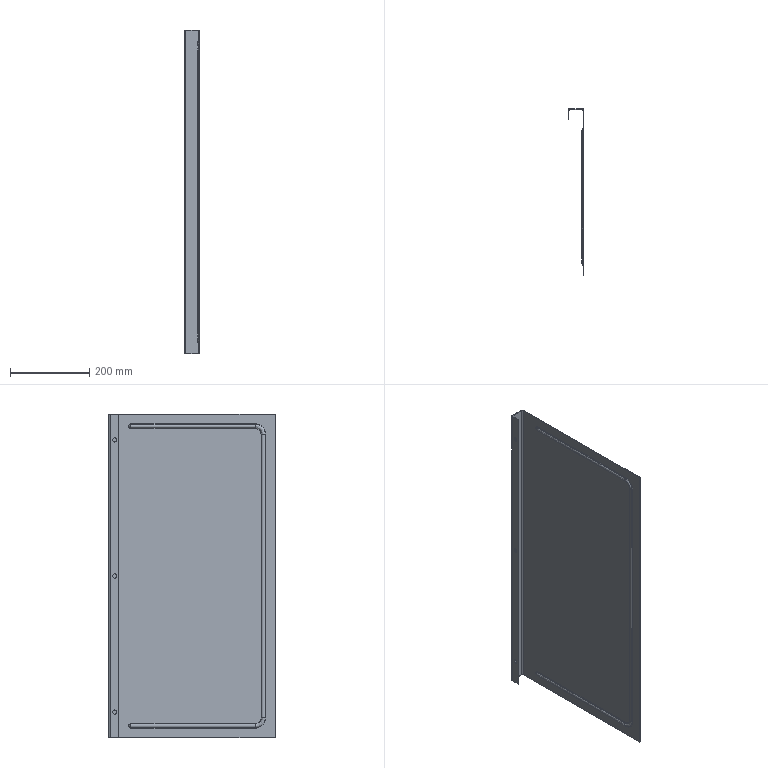Part | STEP file | 750078276 | 1 solid | 58 faces | box 40 x 420 x 817 mm | volume 786846 mm3 | cylinder 28 | spline 20 | plane 10 | commonest cylinder face diameters 4 x8 8 x8 10.5 x6 6 x3 10 x3